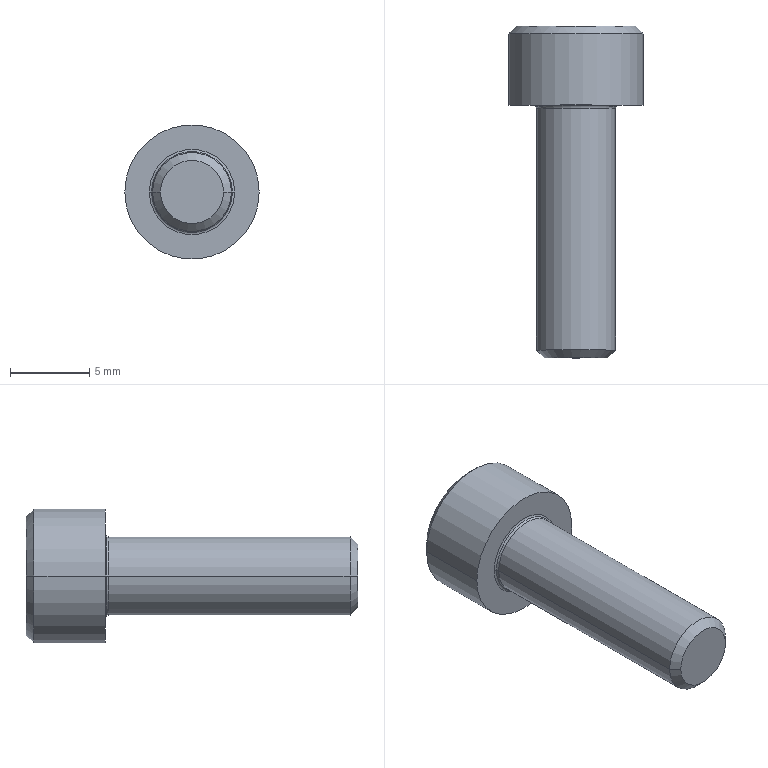Part | Creo | 1 solid | 23 faces | box 8.5 x 21 x 8.5 mm | volume 551.098 mm3 | plane 9 | cone 6 | cylinder 4 | torus 4 | commonest cylinder face diameters 5 x2 8.5 x2
STEP:
#1=CARTESIAN_POINT('',(-215.868,386.495,-46.));
#2=VERTEX_POINT('',#1);
#3=CARTESIAN_POINT('',(-217.022,386.495,-48.));
#4=VERTEX_POINT('',#3);
#5=CARTESIAN_POINT('',(-215.868,386.495,-46.));
#6=CARTESIAN_POINT('',(-215.921,386.464,-46.093));
#7=CARTESIAN_POINT('',(-216.029,386.408,-46.28));
#8=CARTESIAN_POINT('',(-216.195,386.347,-46.567));
#9=CARTESIAN_POINT('',(-216.362,386.315,-46.856));
#10=CARTESIAN_POINT('',(-216.529,386.315,-47.146));
#11=CARTESIAN_POINT('',(-216.696,386.348,-47.435));
#12=CARTESIAN_POINT('',(-216.861,386.409,-47.721));
#13=CARTESIAN_POINT('',(-216.969,386.464,-47.907));
#14=CARTESIAN_POINT('',(-217.022,386.495,-48.));
#15=B_SPLINE_CURVE_WITH_KNOTS('',3,(#5,#6,#7,#8,#9,#10,#11,#12,#13,#14),.UNSPECIFIED.,.F.,.F.,(4,1,1,1,1,1,1,4),(0.,0.1429,0.2857,0.4286,0.5714,0.7143,0.8571,1.),.UNSPECIFIED.);
#16=EDGE_CURVE('',#2,#4,#15,.T.);
#17=ORIENTED_EDGE('',*,*,#16,.F.);
#18=CARTESIAN_POINT('',(-218.177,385.162,-46.));
#19=VERTEX_POINT('',#18);
#20=CARTESIAN_POINT('',(-218.177,385.162,-46.));
#21=DIRECTION('',(0.866,0.5,0.));
#22=VECTOR('',#21,2.667);
#23=LINE('',#20,#22);
#24=EDGE_CURVE('',#19,#2,#23,.T.);
#25=ORIENTED_EDGE('',*,*,#24,.F.);
#26=CARTESIAN_POINT('',(-220.486,386.495,-46.));
#27=VERTEX_POINT('',#26);
#28=CARTESIAN_POINT('',(-218.177,385.162,-46.));
#29=DIRECTION('',(-0.866,0.5,0.));
#30=VECTOR('',#29,2.667);
#31=LINE('',#28,#30);
#32=EDGE_CURVE('',#19,#27,#31,.T.);
#33=ORIENTED_EDGE('',*,*,#32,.T.);
#34=CARTESIAN_POINT('',(-219.332,386.495,-48.));
#35=VERTEX_POINT('',#34);
#36=CARTESIAN_POINT('',(-219.332,386.495,-48.));
#37=CARTESIAN_POINT('',(-219.385,386.464,-47.907));
#38=CARTESIAN_POINT('',(-219.494,386.408,-47.72));
#39=CARTESIAN_POINT('',(-219.659,386.347,-47.433));
#40=CARTESIAN_POINT('',(-219.826,386.315,-47.144));
#41=CARTESIAN_POINT('',(-219.993,386.315,-46.854));
#42=CARTESIAN_POINT('',(-220.16,386.348,-46.565));
#43=CARTESIAN_POINT('',(-220.325,386.409,-46.279));
#44=CARTESIAN_POINT('',(-220.433,386.464,-46.093));
#45=CARTESIAN_POINT('',(-220.486,386.495,-46.));
#46=B_SPLINE_CURVE_WITH_KNOTS('',3,(#36,#37,#38,#39,#40,#41,#42,#43,#44,#45),.UNSPECIFIED.,.F.,.F.,(4,1,1,1,1,1,1,4),(0.,0.1429,0.2857,0.4286,0.5714,0.7143,0.8571,1.),.UNSPECIFIED.);
#47=EDGE_CURVE('',#35,#27,#46,.T.);
#48=ORIENTED_EDGE('',*,*,#47,.F.);
#49=CARTESIAN_POINT('',(-217.022,386.495,-48.));
#50=CARTESIAN_POINT('',(-217.085,386.477,-48.));
#51=CARTESIAN_POINT('',(-217.207,386.444,-48.));
#52=CARTESIAN_POINT('',(-217.384,386.403,-48.));
#53=CARTESIAN_POINT('',(-217.558,386.369,-48.));
#54=CARTESIAN_POINT('',(-217.732,386.343,-48.));
#55=CARTESIAN_POINT('',(-217.909,386.326,-48.));
#56=CARTESIAN_POINT('',(-218.087,386.316,-48.));
#57=CARTESIAN_POINT('',(-218.267,386.316,-48.));
#58=CARTESIAN_POINT('',(-218.445,386.326,-48.));
#59=CARTESIAN_POINT('',(-218.622,386.343,-48.));
#60=CARTESIAN_POINT('',(-218.796,386.369,-48.));
#61=CARTESIAN_POINT('',(-218.97,386.403,-48.));
#62=CARTESIAN_POINT('',(-219.147,386.444,-48.));
#63=CARTESIAN_POINT('',(-219.269,386.477,-48.));
#64=CARTESIAN_POINT('',(-219.332,386.495,-48.));
#65=B_SPLINE_CURVE_WITH_KNOTS('',3,(#49,#50,#51,#52,#53,#54,#55,#56,#57,#58,#59,#60,#61,#62,#63,#64),.UNSPECIFIED.,.F.,.F.,(4,1,1,1,1,1,1,1,1,1,1,1,1,4),(0.,0.07692,0.1538,0.2308,0.3077,0.3846,0.4615,0.5385,0.6154,0.6923,0.7692,0.8462,0.9231,1.),.UNSPECIFIED.);
#66=EDGE_CURVE('',#4,#35,#65,.T.);
#67=ORIENTED_EDGE('',*,*,#66,.F.);
#68=EDGE_LOOP('',(#17,#25,#33,#48,#67));
#69=FACE_OUTER_BOUND('',#68,.F.);
#70=CARTESIAN_POINT('',(-218.177,385.842,-46.));
#71=DIRECTION('',(0.,1.,0.));
#72=DIRECTION('',(1.,0.,0.));
#73=AXIS2_PLACEMENT_3D('',#70,#71,#72);
#74=CONICAL_SURFACE('',#73,1.178,60.);
#75=ADVANCED_FACE('',(#69),#74,.F.);
#76=CARTESIAN_POINT('',(-217.022,388.995,-48.));
#77=VERTEX_POINT('',#76);
#78=CARTESIAN_POINT('',(-215.868,388.995,-46.));
#79=VERTEX_POINT('',#78);
#80=CARTESIAN_POINT('',(-217.022,388.995,-48.));
#81=DIRECTION('',(0.5,0.,0.866));
#82=VECTOR('',#81,2.309);
#83=LINE('',#80,#82);
#84=EDGE_CURVE('',#77,#79,#83,.T.);
#85=ORIENTED_EDGE('',*,*,#84,.T.);
#86=CARTESIAN_POINT('',(-215.868,388.995,-46.));
#87=DIRECTION('',(0.,-1.,0.));
#88=VECTOR('',#87,2.5);
#89=LINE('',#86,#88);
#90=EDGE_CURVE('',#79,#2,#89,.T.);
#91=ORIENTED_EDGE('',*,*,#90,.T.);
#92=ORIENTED_EDGE('',*,*,#16,.T.);
#93=CARTESIAN_POINT('',(-217.022,388.995,-48.));
#94=DIRECTION('',(0.,-1.,0.));
#95=VECTOR('',#94,2.5);
#96=LINE('',#93,#95);
#97=EDGE_CURVE('',#77,#4,#96,.T.);
#98=ORIENTED_EDGE('',*,*,#97,.F.);
#99=EDGE_LOOP('',(#85,#91,#92,#98));
#100=FACE_OUTER_BOUND('',#99,.F.);
#101=CARTESIAN_POINT('',(-217.022,386.495,-48.));
#102=DIRECTION('',(-0.866,0.,0.5));
#103=DIRECTION('',(0.5,0.,0.866));
#104=AXIS2_PLACEMENT_3D('',#101,#102,#103);
#105=PLANE('',#104);
#106=ADVANCED_FACE('',(#100),#105,.T.);
#107=CARTESIAN_POINT('',(-214.427,388.995,-46.));
#108=VERTEX_POINT('',#107);
#109=CARTESIAN_POINT('',(-221.927,388.995,-46.));
#110=VERTEX_POINT('',#109);
#111=CARTESIAN_POINT('',(-218.177,388.995,-46.));
#112=DIRECTION('',(0.,1.,0.));
#113=DIRECTION('',(1.,0.,0.));
#114=AXIS2_PLACEMENT_3D('',#111,#112,#113);
#115=CIRCLE('',#114,3.75);
#116=EDGE_CURVE('',#108,#110,#115,.T.);
#117=ORIENTED_EDGE('',*,*,#116,.F.);
#118=CARTESIAN_POINT('',(-218.177,388.995,-46.));
#119=DIRECTION('',(0.,1.,0.));
#120=DIRECTION('',(-1.,0.,0.));
#121=AXIS2_PLACEMENT_3D('',#118,#119,#120);
#122=CIRCLE('',#121,3.75);
#123=EDGE_CURVE('',#110,#108,#122,.T.);
#124=ORIENTED_EDGE('',*,*,#123,.F.);
#125=EDGE_LOOP('',(#117,#124));
#126=FACE_OUTER_BOUND('',#125,.F.);
#127=CARTESIAN_POINT('',(-217.022,388.995,-44.));
#128=VERTEX_POINT('',#127);
#129=CARTESIAN_POINT('',(-215.868,388.995,-46.));
#130=DIRECTION('',(-0.5,0.,0.866));
#131=VECTOR('',#130,2.309);
#132=LINE('',#129,#131);
#133=EDGE_CURVE('',#79,#128,#132,.T.);
#134=ORIENTED_EDGE('',*,*,#133,.F.);
#135=ORIENTED_EDGE('',*,*,#84,.F.);
#136=CARTESIAN_POINT('',(-219.332,388.995,-48.));
#137=VERTEX_POINT('',#136);
#138=CARTESIAN_POINT('',(-217.022,388.995,-48.));
#139=DIRECTION('',(-1.,0.,0.));
#140=VECTOR('',#139,2.309);
#141=LINE('',#138,#140);
#142=EDGE_CURVE('',#77,#137,#141,.T.);
#143=ORIENTED_EDGE('',*,*,#142,.T.);
#144=CARTESIAN_POINT('',(-220.486,388.995,-46.));
#145=VERTEX_POINT('',#144);
#146=CARTESIAN_POINT('',(-220.486,388.995,-46.));
#147=DIRECTION('',(0.5,0.,-0.866));
#148=VECTOR('',#147,2.309);
#149=LINE('',#146,#148);
#150=EDGE_CURVE('',#145,#137,#149,.T.);
#151=ORIENTED_EDGE('',*,*,#150,.F.);
#152=CARTESIAN_POINT('',(-219.332,388.995,-44.));
#153=VERTEX_POINT('',#152);
#154=CARTESIAN_POINT('',(-219.332,388.995,-44.));
#155=DIRECTION('',(-0.5,0.,-0.866));
#156=VECTOR('',#155,2.309);
#157=LINE('',#154,#156);
#158=EDGE_CURVE('',#153,#145,#157,.T.);
#159=ORIENTED_EDGE('',*,*,#158,.F.);
#160=CARTESIAN_POINT('',(-219.332,388.995,-44.));
#161=DIRECTION('',(1.,0.,0.));
#162=VECTOR('',#161,2.309);
#163=LINE('',#160,#162);
#164=EDGE_CURVE('',#153,#128,#163,.T.);
#165=ORIENTED_EDGE('',*,*,#164,.T.);
#166=EDGE_LOOP('',(#134,#135,#143,#151,#159,#165));
#167=FACE_BOUND('',#166,.F.);
#168=CARTESIAN_POINT('',(-218.177,388.995,-46.));
#169=DIRECTION('',(0.,1.,0.));
#170=DIRECTION('',(1.,0.,0.));
#171=AXIS2_PLACEMENT_3D('',#168,#169,#170);
#172=PLANE('',#171);
#173=ADVANCED_FACE('',(#126,#167),#172,.T.);
#174=CARTESIAN_POINT('',(-213.927,388.495,-46.));
#175=VERTEX_POINT('',#174);
#176=CARTESIAN_POINT('',(-222.427,388.495,-46.));
#177=VERTEX_POINT('',#176);
#178=CARTESIAN_POINT('',(-218.177,388.495,-46.));
#179=DIRECTION('',(0.,1.,0.));
#180=DIRECTION('',(1.,0.,0.));
#181=AXIS2_PLACEMENT_3D('',#178,#179,#180);
#182=CIRCLE('',#181,4.25);
#183=EDGE_CURVE('',#175,#177,#182,.T.);
#184=ORIENTED_EDGE('',*,*,#183,.F.);
#185=CARTESIAN_POINT('',(-214.427,388.995,-46.));
#186=DIRECTION('',(0.7071,-0.7071,0.));
#187=VECTOR('',#186,0.7071);
#188=LINE('',#185,#187);
#189=EDGE_CURVE('',#108,#175,#188,.T.);
#190=ORIENTED_EDGE('',*,*,#189,.F.);
#191=ORIENTED_EDGE('',*,*,#116,.T.);
#192=CARTESIAN_POINT('',(-221.927,388.995,-46.));
#193=DIRECTION('',(-0.7071,-0.7071,0.));
#194=VECTOR('',#193,0.7071);
#195=LINE('',#192,#194);
#196=EDGE_CURVE('',#110,#177,#195,.T.);
#197=ORIENTED_EDGE('',*,*,#196,.T.);
#198=EDGE_LOOP('',(#184,#190,#191,#197));
#199=FACE_OUTER_BOUND('',#198,.F.);
#200=CARTESIAN_POINT('',(-218.177,388.745,-46.));
#201=DIRECTION('',(0.,-1.,0.));
#202=DIRECTION('',(-1.,0.,0.));
#203=AXIS2_PLACEMENT_3D('',#200,#201,#202);
#204=CONICAL_SURFACE('',#203,4.,45.);
#205=ADVANCED_FACE('',(#199),#204,.T.);
#206=ORIENTED_EDGE('',*,*,#183,.T.);
#207=CARTESIAN_POINT('',(-222.427,383.995,-46.));
#208=VERTEX_POINT('',#207);
#209=CARTESIAN_POINT('',(-222.427,383.995,-46.));
#210=DIRECTION('',(0.,1.,0.));
#211=VECTOR('',#210,4.5);
#212=LINE('',#209,#211);
#213=EDGE_CURVE('',#208,#177,#212,.T.);
#214=ORIENTED_EDGE('',*,*,#213,.F.);
#215=CARTESIAN_POINT('',(-213.927,383.995,-46.));
#216=VERTEX_POINT('',#215);
#217=CARTESIAN_POINT('',(-218.177,383.995,-46.));
#218=DIRECTION('',(0.,-1.,0.));
#219=DIRECTION('',(-1.,0.,0.));
#220=AXIS2_PLACEMENT_3D('',#217,#218,#219);
#221=CIRCLE('',#220,4.25);
#222=EDGE_CURVE('',#208,#216,#221,.T.);
#223=ORIENTED_EDGE('',*,*,#222,.T.);
#224=CARTESIAN_POINT('',(-213.927,383.995,-46.));
#225=DIRECTION('',(0.,1.,0.));
#226=VECTOR('',#225,4.5);
#227=LINE('',#224,#226);
#228=EDGE_CURVE('',#216,#175,#227,.T.);
#229=ORIENTED_EDGE('',*,*,#228,.T.);
#230=EDGE_LOOP('',(#206,#214,#223,#229));
#231=FACE_OUTER_BOUND('',#230,.F.);
#232=CARTESIAN_POINT('',(-218.177,383.995,-46.));
#233=DIRECTION('',(0.,1.,0.));
#234=DIRECTION('',(1.,0.,0.));
#235=AXIS2_PLACEMENT_3D('',#232,#233,#234);
#236=CYLINDRICAL_SURFACE('',#235,4.25);
#237=ADVANCED_FACE('',(#231),#236,.T.);
#238=CARTESIAN_POINT('',(-218.177,388.495,-46.));
#239=DIRECTION('',(0.,1.,0.));
#240=DIRECTION('',(-1.,0.,0.));
#241=AXIS2_PLACEMENT_3D('',#238,#239,#240);
#242=CIRCLE('',#241,4.25);
#243=EDGE_CURVE('',#177,#175,#242,.T.);
#244=ORIENTED_EDGE('',*,*,#243,.T.);
#245=ORIENTED_EDGE('',*,*,#228,.F.);
#246=CARTESIAN_POINT('',(-218.177,383.995,-46.));
#247=DIRECTION('',(0.,-1.,0.));
#248=DIRECTION('',(1.,0.,0.));
#249=AXIS2_PLACEMENT_3D('',#246,#247,#248);
#250=CIRCLE('',#249,4.25);
#251=EDGE_CURVE('',#216,#208,#250,.T.);
#252=ORIENTED_EDGE('',*,*,#251,.T.);
#253=ORIENTED_EDGE('',*,*,#213,.T.);
#254=EDGE_LOOP('',(#244,#245,#252,#253));
#255=FACE_OUTER_BOUND('',#254,.F.);
#256=CARTESIAN_POINT('',(-218.177,383.995,-46.));
#257=DIRECTION('',(0.,1.,0.));
#258=DIRECTION('',(1.,0.,0.));
#259=AXIS2_PLACEMENT_3D('',#256,#257,#258);
#260=CYLINDRICAL_SURFACE('',#259,4.25);
#261=ADVANCED_FACE('',(#255),#260,.T.);
#262=ORIENTED_EDGE('',*,*,#243,.F.);
#263=ORIENTED_EDGE('',*,*,#196,.F.);
#264=ORIENTED_EDGE('',*,*,#123,.T.);
#265=ORIENTED_EDGE('',*,*,#189,.T.);
#266=EDGE_LOOP('',(#262,#263,#264,#265));
#267=FACE_OUTER_BOUND('',#266,.F.);
#268=CARTESIAN_POINT('',(-218.177,388.745,-46.));
#269=DIRECTION('',(0.,-1.,0.));
#270=DIRECTION('',(-1.,0.,0.));
#271=AXIS2_PLACEMENT_3D('',#268,#269,#270);
#272=CONICAL_SURFACE('',#271,4.,45.);
#273=ADVANCED_FACE('',(#267),#272,.T.);
#274=ORIENTED_EDGE('',*,*,#251,.F.);
#275=ORIENTED_EDGE('',*,*,#222,.F.);
#276=EDGE_LOOP('',(#274,#275));
#277=FACE_OUTER_BOUND('',#276,.F.);
#278=CARTESIAN_POINT('',(-215.477,383.995,-46.));
#279=VERTEX_POINT('',#278);
#280=CARTESIAN_POINT('',(-220.877,383.995,-46.));
#281=VERTEX_POINT('',#280);
#282=CARTESIAN_POINT('',(-218.177,383.995,-46.));
#283=DIRECTION('',(0.,1.,0.));
#284=DIRECTION('',(1.,0.,0.));
#285=AXIS2_PLACEMENT_3D('',#282,#283,#284);
#286=CIRCLE('',#285,2.7);
#287=EDGE_CURVE('',#279,#281,#286,.T.);
#288=ORIENTED_EDGE('',*,*,#287,.F.);
#289=CARTESIAN_POINT('',(-218.177,383.995,-46.));
#290=DIRECTION('',(0.,1.,0.));
#291=DIRECTION('',(-1.,0.,0.));
#292=AXIS2_PLACEMENT_3D('',#289,#290,#291);
#293=CIRCLE('',#292,2.7);
#294=EDGE_CURVE('',#281,#279,#293,.T.);
#295=ORIENTED_EDGE('',*,*,#294,.F.);
#296=EDGE_LOOP('',(#288,#295));
#297=FACE_BOUND('',#296,.F.);
#298=CARTESIAN_POINT('',(-218.177,383.995,-46.));
#299=DIRECTION('',(0.,1.,0.));
#300=DIRECTION('',(1.,0.,0.));
#301=AXIS2_PLACEMENT_3D('',#298,#299,#300);
#302=PLANE('',#301);
#303=ADVANCED_FACE('',(#277,#297),#302,.F.);
#304=ORIENTED_EDGE('',*,*,#287,.T.);
#305=CARTESIAN_POINT('',(-220.736,383.937,-46.));
#306=VERTEX_POINT('',#305);
#307=CARTESIAN_POINT('',(-220.877,383.795,-46.));
#308=DIRECTION('',(0.,0.,-1.));
#309=DIRECTION('',(0.,1.,0.));
#310=AXIS2_PLACEMENT_3D('',#307,#308,#309);
#311=CIRCLE('',#310,0.2);
#312=EDGE_CURVE('',#281,#306,#311,.T.);
#313=ORIENTED_EDGE('',*,*,#312,.T.);
#314=CARTESIAN_POINT('',(-215.618,383.937,-46.));
#315=VERTEX_POINT('',#314);
#316=CARTESIAN_POINT('',(-218.177,383.937,-46.));
#317=DIRECTION('',(0.,1.,0.));
#318=DIRECTION('',(1.,0.,0.));
#319=AXIS2_PLACEMENT_3D('',#316,#317,#318);
#320=CIRCLE('',#319,2.559);
#321=EDGE_CURVE('',#315,#306,#320,.T.);
#322=ORIENTED_EDGE('',*,*,#321,.F.);
#323=CARTESIAN_POINT('',(-215.477,383.795,-46.));
#324=DIRECTION('',(0.,0.,1.));
#325=DIRECTION('',(0.,1.,0.));
#326=AXIS2_PLACEMENT_3D('',#323,#324,#325);
#327=CIRCLE('',#326,0.2);
#328=EDGE_CURVE('',#279,#315,#327,.T.);
#329=ORIENTED_EDGE('',*,*,#328,.F.);
#330=EDGE_LOOP('',(#304,#313,#322,#329));
#331=FACE_OUTER_BOUND('',#330,.F.);
#332=CARTESIAN_POINT('',(-218.177,383.795,-46.));
#333=DIRECTION('',(0.,1.,0.));
#334=DIRECTION('',(1.,0.,0.));
#335=AXIS2_PLACEMENT_3D('',#332,#333,#334);
#336=TOROIDAL_SURFACE('',#335,2.7,0.2);
#337=ADVANCED_FACE('',(#331),#336,.F.);
#338=ORIENTED_EDGE('',*,*,#294,.T.);
#339=ORIENTED_EDGE('',*,*,#328,.T.);
#340=CARTESIAN_POINT('',(-218.177,383.937,-46.));
#341=DIRECTION('',(0.,1.,0.));
#342=DIRECTION('',(-1.,0.,0.));
#343=AXIS2_PLACEMENT_3D('',#340,#341,#342);
#344=CIRCLE('',#343,2.559);
#345=EDGE_CURVE('',#306,#315,#344,.T.);
#346=ORIENTED_EDGE('',*,*,#345,.F.);
#347=ORIENTED_EDGE('',*,*,#312,.F.);
#348=EDGE_LOOP('',(#338,#339,#346,#347));
#349=FACE_OUTER_BOUND('',#348,.F.);
#350=CARTESIAN_POINT('',(-218.177,383.795,-46.));
#351=DIRECTION('',(0.,1.,0.));
#352=DIRECTION('',(1.,0.,0.));
#353=AXIS2_PLACEMENT_3D('',#350,#351,#352);
#354=TOROIDAL_SURFACE('',#353,2.7,0.2);
#355=ADVANCED_FACE('',(#349),#354,.F.);
#356=CARTESIAN_POINT('',(-220.677,383.795,-46.));
#357=VERTEX_POINT('',#356);
#358=CARTESIAN_POINT('',(-215.677,383.795,-46.));
#359=VERTEX_POINT('',#358);
#360=CARTESIAN_POINT('',(-218.177,383.795,-46.));
#361=DIRECTION('',(0.,1.,0.));
#362=DIRECTION('',(-1.,0.,0.));
#363=AXIS2_PLACEMENT_3D('',#360,#361,#362);
#364=CIRCLE('',#363,2.5);
#365=EDGE_CURVE('',#357,#359,#364,.T.);
#366=ORIENTED_EDGE('',*,*,#365,.F.);
#367=CARTESIAN_POINT('',(-220.877,383.795,-46.));
#368=DIRECTION('',(0.,0.,-1.));
#369=DIRECTION('',(0.7071,0.7071,0.));
#370=AXIS2_PLACEMENT_3D('',#367,#368,#369);
#371=CIRCLE('',#370,0.2);
#372=EDGE_CURVE('',#306,#357,#371,.T.);
#373=ORIENTED_EDGE('',*,*,#372,.F.);
#374=ORIENTED_EDGE('',*,*,#345,.T.);
#375=CARTESIAN_POINT('',(-215.477,383.795,-46.));
#376=DIRECTION('',(0.,0.,1.));
#377=DIRECTION('',(-0.7071,0.7071,0.));
#378=AXIS2_PLACEMENT_3D('',#375,#376,#377);
#379=CIRCLE('',#378,0.2);
#380=EDGE_CURVE('',#315,#359,#379,.T.);
#381=ORIENTED_EDGE('',*,*,#380,.T.);
#382=EDGE_LOOP('',(#366,#373,#374,#381));
#383=FACE_OUTER_BOUND('',#382,.F.);
#384=CARTESIAN_POINT('',(-218.177,383.795,-46.));
#385=DIRECTION('',(0.,1.,0.));
#386=DIRECTION('',(1.,0.,0.));
#387=AXIS2_PLACEMENT_3D('',#384,#385,#386);
#388=TOROIDAL_SURFACE('',#387,2.7,0.2);
#389=ADVANCED_FACE('',(#383),#388,.F.);
#390=CARTESIAN_POINT('',(-215.677,368.495,-46.));
#391=VERTEX_POINT('',#390);
#392=CARTESIAN_POINT('',(-220.677,368.495,-46.));
#393=VERTEX_POINT('',#392);
#394=CARTESIAN_POINT('',(-218.177,368.495,-46.));
#395=DIRECTION('',(0.,-1.,0.));
#396=DIRECTION('',(1.,0.,0.));
#397=AXIS2_PLACEMENT_3D('',#394,#395,#396);
#398=CIRCLE('',#397,2.5);
#399=EDGE_CURVE('',#391,#393,#398,.T.);
#400=ORIENTED_EDGE('',*,*,#399,.T.);
#401=CARTESIAN_POINT('',(-220.677,368.495,-46.));
#402=DIRECTION('',(0.,1.,0.));
#403=VECTOR('',#402,15.3);
#404=LINE('',#401,#403);
#405=EDGE_CURVE('',#393,#357,#404,.T.);
#406=ORIENTED_EDGE('',*,*,#405,.T.);
#407=ORIENTED_EDGE('',*,*,#365,.T.);
#408=CARTESIAN_POINT('',(-215.677,368.495,-46.));
#409=DIRECTION('',(0.,1.,0.));
#410=VECTOR('',#409,15.3);
#411=LINE('',#408,#410);
#412=EDGE_CURVE('',#391,#359,#411,.T.);
#413=ORIENTED_EDGE('',*,*,#412,.F.);
#414=EDGE_LOOP('',(#400,#406,#407,#413));
#415=FACE_OUTER_BOUND('',#414,.F.);
#416=CARTESIAN_POINT('',(-218.177,367.995,-46.));
#417=DIRECTION('',(0.,1.,0.));
#418=DIRECTION('',(1.,0.,0.));
#419=AXIS2_PLACEMENT_3D('',#416,#417,#418);
#420=CYLINDRICAL_SURFACE('',#419,2.5);
#421=ADVANCED_FACE('',(#415),#420,.T.);
#422=CARTESIAN_POINT('',(-216.177,367.995,-46.));
#423=VERTEX_POINT('',#422);
#424=CARTESIAN_POINT('',(-220.177,367.995,-46.));
#425=VERTEX_POINT('',#424);
#426=CARTESIAN_POINT('',(-218.177,367.995,-46.));
#427=DIRECTION('',(0.,-1.,0.));
#428=DIRECTION('',(1.,0.,0.));
#429=AXIS2_PLACEMENT_3D('',#426,#427,#428);
#430=CIRCLE('',#429,2.);
#431=EDGE_CURVE('',#423,#425,#430,.T.);
#432=ORIENTED_EDGE('',*,*,#431,.T.);
#433=CARTESIAN_POINT('',(-220.177,367.995,-46.));
#434=DIRECTION('',(-0.7071,0.7071,0.));
#435=VECTOR('',#434,0.7071);
#436=LINE('',#433,#435);
#437=EDGE_CURVE('',#425,#393,#436,.T.);
#438=ORIENTED_EDGE('',*,*,#437,.T.);
#439=ORIENTED_EDGE('',*,*,#399,.F.);
#440=CARTESIAN_POINT('',(-216.177,367.995,-46.));
#441=DIRECTION('',(0.7071,0.7071,0.));
#442=VECTOR('',#441,0.7071);
#443=LINE('',#440,#442);
#444=EDGE_CURVE('',#423,#391,#443,.T.);
#445=ORIENTED_EDGE('',*,*,#444,.F.);
#446=EDGE_LOOP('',(#432,#438,#439,#445));
#447=FACE_OUTER_BOUND('',#446,.F.);
#448=CARTESIAN_POINT('',(-218.177,368.245,-46.));
#449=DIRECTION('',(0.,1.,0.));
#450=DIRECTION('',(1.,0.,0.));
#451=AXIS2_PLACEMENT_3D('',#448,#449,#450);
#452=CONICAL_SURFACE('',#451,2.25,45.);
#453=ADVANCED_FACE('',(#447),#452,.T.);
#454=ORIENTED_EDGE('',*,*,#431,.F.);
#455=CARTESIAN_POINT('',(-218.177,367.995,-46.));
#456=DIRECTION('',(0.,-1.,0.));
#457=DIRECTION('',(-1.,0.,0.));
#458=AXIS2_PLACEMENT_3D('',#455,#456,#457);
#459=CIRCLE('',#458,2.);
#460=EDGE_CURVE('',#425,#423,#459,.T.);
#461=ORIENTED_EDGE('',*,*,#460,.F.);
#462=EDGE_LOOP('',(#454,#461));
#463=FACE_OUTER_BOUND('',#462,.F.);
#464=CARTESIAN_POINT('',(-218.177,367.995,-46.));
#465=DIRECTION('',(0.,1.,0.));
#466=DIRECTION('',(1.,0.,0.));
#467=AXIS2_PLACEMENT_3D('',#464,#465,#466);
#468=PLANE('',#467);
#469=ADVANCED_FACE('',(#463),#468,.F.);
#470=ORIENTED_EDGE('',*,*,#460,.T.);
#471=ORIENTED_EDGE('',*,*,#444,.T.);
#472=CARTESIAN_POINT('',(-218.177,368.495,-46.));
#473=DIRECTION('',(0.,-1.,0.));
#474=DIRECTION('',(-1.,0.,0.));
#475=AXIS2_PLACEMENT_3D('',#472,#473,#474);
#476=CIRCLE('',#475,2.5);
#477=EDGE_CURVE('',#393,#391,#476,.T.);
#478=ORIENTED_EDGE('',*,*,#477,.F.);
#479=ORIENTED_EDGE('',*,*,#437,.F.);
#480=EDGE_LOOP('',(#470,#471,#478,#479));
#481=FACE_OUTER_BOUND('',#480,.F.);
#482=CARTESIAN_POINT('',(-218.177,368.245,-46.));
#483=DIRECTION('',(0.,1.,0.));
#484=DIRECTION('',(1.,0.,0.));
#485=AXIS2_PLACEMENT_3D('',#482,#483,#484);
#486=CONICAL_SURFACE('',#485,2.25,45.);
#487=ADVANCED_FACE('',(#481),#486,.T.);
#488=ORIENTED_EDGE('',*,*,#477,.T.);
#489=ORIENTED_EDGE('',*,*,#412,.T.);
#490=CARTESIAN_POINT('',(-218.177,383.795,-46.));
#491=DIRECTION('',(0.,1.,0.));
#492=DIRECTION('',(1.,0.,0.));
#493=AXIS2_PLACEMENT_3D('',#490,#491,#492);
#494=CIRCLE('',#493,2.5);
#495=EDGE_CURVE('',#359,#357,#494,.T.);
#496=ORIENTED_EDGE('',*,*,#495,.T.);
#497=ORIENTED_EDGE('',*,*,#405,.F.);
#498=EDGE_LOOP('',(#488,#489,#496,#497));
#499=FACE_OUTER_BOUND('',#498,.F.);
#500=CARTESIAN_POINT('',(-218.177,367.995,-46.));
#501=DIRECTION('',(0.,1.,0.));
#502=DIRECTION('',(1.,0.,0.));
#503=AXIS2_PLACEMENT_3D('',#500,#501,#502);
#504=CYLINDRICAL_SURFACE('',#503,2.5);
#505=ADVANCED_FACE('',(#499),#504,.T.);
#506=ORIENTED_EDGE('',*,*,#495,.F.);
#507=ORIENTED_EDGE('',*,*,#380,.F.);
#508=ORIENTED_EDGE('',*,*,#321,.T.);
#509=ORIENTED_EDGE('',*,*,#372,.T.);
#510=EDGE_LOOP('',(#506,#507,#508,#509));
#511=FACE_OUTER_BOUND('',#510,.F.);
#512=CARTESIAN_POINT('',(-218.177,383.795,-46.));
#513=DIRECTION('',(0.,1.,0.));
#514=DIRECTION('',(1.,0.,0.));
#515=AXIS2_PLACEMENT_3D('',#512,#513,#514);
#516=TOROIDAL_SURFACE('',#515,2.7,0.2);
#517=ADVANCED_FACE('',(#511),#516,.F.);
#518=ORIENTED_EDGE('',*,*,#133,.T.);
#519=CARTESIAN_POINT('',(-217.022,386.495,-44.));
#520=VERTEX_POINT('',#519);
#521=CARTESIAN_POINT('',(-217.022,388.995,-44.));
#522=DIRECTION('',(0.,-1.,0.));
#523=VECTOR('',#522,2.5);
#524=LINE('',#521,#523);
#525=EDGE_CURVE('',#128,#520,#524,.T.);
#526=ORIENTED_EDGE('',*,*,#525,.T.);
#527=CARTESIAN_POINT('',(-217.022,386.495,-44.));
#528=CARTESIAN_POINT('',(-216.969,386.464,-44.093));
#529=CARTESIAN_POINT('',(-216.86,386.408,-44.28));
#530=CARTESIAN_POINT('',(-216.695,386.347,-44.567));
#531=CARTESIAN_POINT('',(-216.528,386.315,-44.856));
#532=CARTESIAN_POINT('',(-216.361,386.315,-45.146));
#533=CARTESIAN_POINT('',(-216.194,386.348,-45.435));
#534=CARTESIAN_POINT('',(-216.029,386.409,-45.721));
#535=CARTESIAN_POINT('',(-215.921,386.464,-45.907));
#536=CARTESIAN_POINT('',(-215.868,386.495,-46.));
#537=B_SPLINE_CURVE_WITH_KNOTS('',3,(#527,#528,#529,#530,#531,#532,#533,#534,#535,#536),.UNSPECIFIED.,.F.,.F.,(4,1,1,1,1,1,1,4),(0.,0.1429,0.2857,0.4286,0.5714,0.7143,0.8571,1.),.UNSPECIFIED.);
#538=EDGE_CURVE('',#520,#2,#537,.T.);
#539=ORIENTED_EDGE('',*,*,#538,.T.);
#540=ORIENTED_EDGE('',*,*,#90,.F.);
#541=EDGE_LOOP('',(#518,#526,#539,#540));
#542=FACE_OUTER_BOUND('',#541,.F.);
#543=CARTESIAN_POINT('',(-215.868,386.495,-46.));
#544=DIRECTION('',(-0.866,0.,-0.5));
#545=DIRECTION('',(-0.5,0.,0.866));
#546=AXIS2_PLACEMENT_3D('',#543,#544,#545);
#547=PLANE('',#546);
#548=ADVANCED_FACE('',(#542),#547,.T.);
#549=ORIENTED_EDGE('',*,*,#164,.F.);
#550=CARTESIAN_POINT('',(-219.332,386.495,-44.));
#551=VERTEX_POINT('',#550);
#552=CARTESIAN_POINT('',(-219.332,388.995,-44.));
#553=DIRECTION('',(0.,-1.,0.));
#554=VECTOR('',#553,2.5);
#555=LINE('',#552,#554);
#556=EDGE_CURVE('',#153,#551,#555,.T.);
#557=ORIENTED_EDGE('',*,*,#556,.T.);
#558=CARTESIAN_POINT('',(-219.332,386.495,-44.));
#559=CARTESIAN_POINT('',(-219.269,386.477,-44.));
#560=CARTESIAN_POINT('',(-219.147,386.444,-44.));
#561=CARTESIAN_POINT('',(-218.97,386.403,-44.));
#562=CARTESIAN_POINT('',(-218.796,386.369,-44.));
#563=CARTESIAN_POINT('',(-218.622,386.343,-44.));
#564=CARTESIAN_POINT('',(-218.445,386.326,-44.));
#565=CARTESIAN_POINT('',(-218.267,386.316,-44.));
#566=CARTESIAN_POINT('',(-218.087,386.316,-44.));
#567=CARTESIAN_POINT('',(-217.909,386.326,-44.));
#568=CARTESIAN_POINT('',(-217.732,386.343,-44.));
#569=CARTESIAN_POINT('',(-217.558,386.369,-44.));
#570=CARTESIAN_POINT('',(-217.384,386.403,-44.));
#571=CARTESIAN_POINT('',(-217.207,386.444,-44.));
#572=CARTESIAN_POINT('',(-217.085,386.477,-44.));
#573=CARTESIAN_POINT('',(-217.022,386.495,-44.));
#574=B_SPLINE_CURVE_WITH_KNOTS('',3,(#558,#559,#560,#561,#562,#563,#564,#565,#566,#567,#568,#569,#570,#571,#572,#573),.UNSPECIFIED.,.F.,.F.,(4,1,1,1,1,1,1,1,1,1,1,1,1,4),(0.,0.07692,0.1538,0.2308,0.3077,0.3846,0.4615,0.5385,0.6154,0.6923,0.7692,0.8462,0.9231,1.),.UNSPECIFIED.);
#575=EDGE_CURVE('',#551,#520,#574,.T.);
#576=ORIENTED_EDGE('',*,*,#575,.T.);
#577=ORIENTED_EDGE('',*,*,#525,.F.);
#578=EDGE_LOOP('',(#549,#557,#576,#577));
#579=FACE_OUTER_BOUND('',#578,.F.);
#580=CARTESIAN_POINT('',(-217.022,386.495,-44.));
#581=DIRECTION('',(0.,0.,-1.));
#582=DIRECTION('',(0.,1.,0.));
#583=AXIS2_PLACEMENT_3D('',#580,#581,#582);
#584=PLANE('',#583);
#585=ADVANCED_FACE('',(#579),#584,.T.);
#586=ORIENTED_EDGE('',*,*,#158,.T.);
#587=CARTESIAN_POINT('',(-220.486,388.995,-46.));
#588=DIRECTION('',(0.,-1.,0.));
#589=VECTOR('',#588,2.5);
#590=LINE('',#587,#589);
#591=EDGE_CURVE('',#145,#27,#590,.T.);
#592=ORIENTED_EDGE('',*,*,#591,.T.);
#593=CARTESIAN_POINT('',(-220.486,386.495,-46.));
#594=CARTESIAN_POINT('',(-220.433,386.464,-45.907));
#595=CARTESIAN_POINT('',(-220.325,386.409,-45.721));
#596=CARTESIAN_POINT('',(-220.16,386.348,-45.435));
#597=CARTESIAN_POINT('',(-219.993,386.315,-45.146));
#598=CARTESIAN_POINT('',(-219.826,386.315,-44.856));
#599=CARTESIAN_POINT('',(-219.659,386.347,-44.567));
#600=CARTESIAN_POINT('',(-219.494,386.408,-44.28));
#601=CARTESIAN_POINT('',(-219.385,386.464,-44.093));
#602=CARTESIAN_POINT('',(-219.332,386.495,-44.));
#603=B_SPLINE_CURVE_WITH_KNOTS('',3,(#593,#594,#595,#596,#597,#598,#599,#600,#601,#602),.UNSPECIFIED.,.F.,.F.,(4,1,1,1,1,1,1,4),(0.,0.1429,0.2857,0.4286,0.5714,0.7143,0.8571,1.),.UNSPECIFIED.);
#604=EDGE_CURVE('',#27,#551,#603,.T.);
#605=ORIENTED_EDGE('',*,*,#604,.T.);
#606=ORIENTED_EDGE('',*,*,#556,.F.);
#607=EDGE_LOOP('',(#586,#592,#605,#606));
#608=FACE_OUTER_BOUND('',#607,.F.);
#609=CARTESIAN_POINT('',(-219.332,386.495,-44.));
#610=DIRECTION('',(0.866,0.,-0.5));
#611=DIRECTION('',(-0.5,0.,-0.866));
#612=AXIS2_PLACEMENT_3D('',#609,#610,#611);
#613=PLANE('',#612);
#614=ADVANCED_FACE('',(#608),#613,.T.);
#615=ORIENTED_EDGE('',*,*,#150,.T.);
#616=CARTESIAN_POINT('',(-219.332,388.995,-48.));
#617=DIRECTION('',(0.,-1.,0.));
#618=VECTOR('',#617,2.5);
#619=LINE('',#616,#618);
#620=EDGE_CURVE('',#137,#35,#619,.T.);
#621=ORIENTED_EDGE('',*,*,#620,.T.);
#622=ORIENTED_EDGE('',*,*,#47,.T.);
#623=ORIENTED_EDGE('',*,*,#591,.F.);
#624=EDGE_LOOP('',(#615,#621,#622,#623));
#625=FACE_OUTER_BOUND('',#624,.F.);
#626=CARTESIAN_POINT('',(-220.486,386.495,-46.));
#627=DIRECTION('',(0.866,0.,0.5));
#628=DIRECTION('',(0.5,0.,-0.866));
#629=AXIS2_PLACEMENT_3D('',#626,#627,#628);
#630=PLANE('',#629);
#631=ADVANCED_FACE('',(#625),#630,.T.);
#632=ORIENTED_EDGE('',*,*,#142,.F.);
#633=ORIENTED_EDGE('',*,*,#97,.T.);
#634=ORIENTED_EDGE('',*,*,#66,.T.);
#635=ORIENTED_EDGE('',*,*,#620,.F.);
#636=EDGE_LOOP('',(#632,#633,#634,#635));
#637=FACE_OUTER_BOUND('',#636,.F.);
#638=CARTESIAN_POINT('',(-219.332,386.495,-48.));
#639=DIRECTION('',(0.,0.,1.));
#640=DIRECTION('',(0.,-1.,0.));
#641=AXIS2_PLACEMENT_3D('',#638,#639,#640);
#642=PLANE('',#641);
#643=ADVANCED_FACE('',(#637),#642,.T.);
#644=ORIENTED_EDGE('',*,*,#604,.F.);
#645=ORIENTED_EDGE('',*,*,#32,.F.);
#646=ORIENTED_EDGE('',*,*,#24,.T.);
#647=ORIENTED_EDGE('',*,*,#538,.F.);
#648=ORIENTED_EDGE('',*,*,#575,.F.);
#649=EDGE_LOOP('',(#644,#645,#646,#647,#648));
#650=FACE_OUTER_BOUND('',#649,.F.);
#651=CARTESIAN_POINT('',(-218.177,385.842,-46.));
#652=DIRECTION('',(0.,1.,0.));
#653=DIRECTION('',(1.,0.,0.));
#654=AXIS2_PLACEMENT_3D('',#651,#652,#653);
#655=CONICAL_SURFACE('',#654,1.178,60.);
#656=ADVANCED_FACE('',(#650),#655,.F.);
#657=CLOSED_SHELL('',(#75,#106,#173,#205,#237,#261,#273,#303,#337,#355,#389,#421,#453,#469,#487,#505,#517,#548,#585,#614,#631,#643,#656));
#658=MANIFOLD_SOLID_BREP('',#657);
#659=(LENGTH_UNIT()NAMED_UNIT(*)SI_UNIT(.MILLI.,.METRE.));
#660=UNCERTAINTY_MEASURE_WITH_UNIT(LENGTH_MEASURE(0.00242),#659,'','');
#661=(NAMED_UNIT(*)PLANE_ANGLE_UNIT()SI_UNIT($,.RADIAN.));
#662=PLANE_ANGLE_MEASURE_WITH_UNIT(PLANE_ANGLE_MEASURE(0.01745),#661);
#663=(CONVERSION_BASED_UNIT('DEGREE',#662)NAMED_UNIT(*)PLANE_ANGLE_UNIT());
#664=(NAMED_UNIT(*)SI_UNIT($,.STERADIAN.)SOLID_ANGLE_UNIT());
#665=(GEOMETRIC_REPRESENTATION_CONTEXT(3)GLOBAL_UNCERTAINTY_ASSIGNED_CONTEXT((#660))GLOBAL_UNIT_ASSIGNED_CONTEXT((#659,#663,#664))REPRESENTATION_CONTEXT('',''));
#666=ADVANCED_BREP_SHAPE_REPRESENTATION('',(#658),#665);